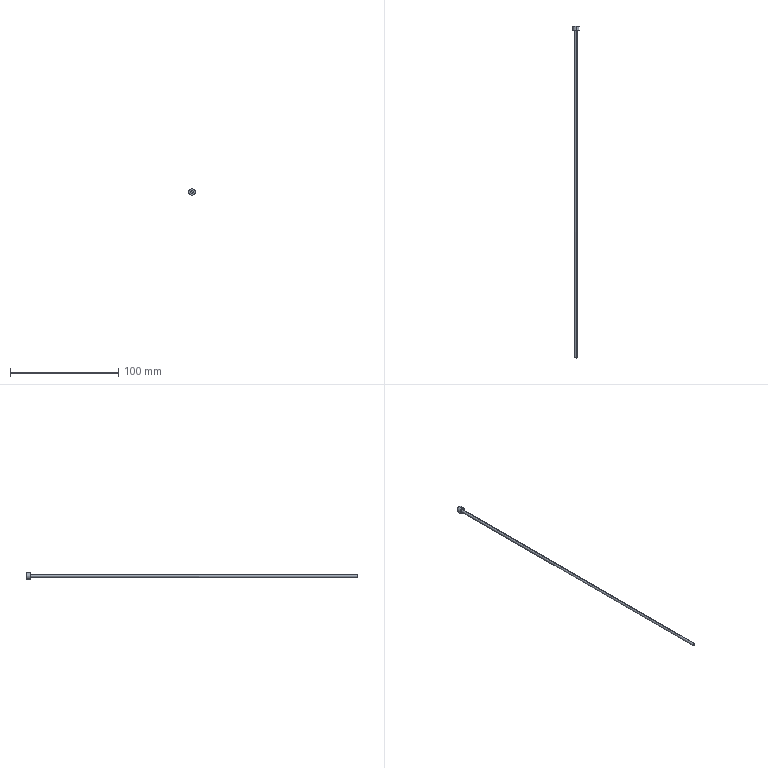Part | STEP file | 1 solid | 7 faces | box 6 x 306.305 x 6 mm | volume 1597 mm3 | cylinder 4 | plane 3 | commonest cylinder face diameters 2.5 x2 6 x2
STEP:
#1=CARTESIAN_POINT('',(0.,0.,0.));
#2=DIRECTION('',(0.,0.,1.));
#3=DIRECTION('',(1.,0.,0.));
#4=AXIS2_PLACEMENT_3D('',#1,#2,#3);
#5=CARTESIAN_POINT('',(-72.862,345.5,129.66));
#6=VERTEX_POINT('',#5);
#7=CARTESIAN_POINT('',(-72.862,345.5,135.66));
#8=VERTEX_POINT('',#7);
#9=CARTESIAN_POINT('',(-72.862,345.5,132.66));
#10=DIRECTION('',(0.,-1.,0.));
#11=DIRECTION('',(0.,0.,-1.));
#12=AXIS2_PLACEMENT_3D('',#9,#10,#11);
#13=CIRCLE('',#12,3.);
#14=CARTESIAN_POINT('',(-72.862,345.5,132.66));
#15=DIRECTION('',(0.,-1.,0.));
#16=DIRECTION('',(0.,0.,-1.));
#17=AXIS2_PLACEMENT_3D('',#14,#15,#16);
#18=CYLINDRICAL_SURFACE('',#17,3.);
#19=CARTESIAN_POINT('',(0.,0.));
#20=DIRECTION('',(1.,0.));
#21=VECTOR('',#20,1.);
#22=LINE('',#19,#21);
#23=(GEOMETRIC_REPRESENTATION_CONTEXT(2)PARAMETRIC_REPRESENTATION_CONTEXT()REPRESENTATION_CONTEXT('',''));
#24=DEFINITIONAL_REPRESENTATION('',(#22),#23);
#25=PCURVE('',#18,#24);
#26=CARTESIAN_POINT('',(-72.862,345.5,110.196));
#27=DIRECTION('',(0.,-1.,0.));
#28=DIRECTION('',(0.,0.,-1.));
#29=AXIS2_PLACEMENT_3D('',#26,#27,#28);
#30=PLANE('',#29);
#31=CARTESIAN_POINT('',(-22.464,-0.000000011));
#32=DIRECTION('',(1.,0.));
#33=AXIS2_PLACEMENT_2D('',#31,#32);
#34=CIRCLE('',#33,3.);
#35=(GEOMETRIC_REPRESENTATION_CONTEXT(2)PARAMETRIC_REPRESENTATION_CONTEXT()REPRESENTATION_CONTEXT('',''));
#36=DEFINITIONAL_REPRESENTATION('',(#34),#35);
#37=PCURVE('',#30,#36);
#38=SURFACE_CURVE('',#13,(#25,#37),.PCURVE_S1.);
#39=EDGE_CURVE('',#6,#8,#38,.T.);
#40=ORIENTED_EDGE('',*,*,#39,.T.);
#41=CARTESIAN_POINT('',(-72.862,341.5,135.66));
#42=VERTEX_POINT('',#41);
#43=CARTESIAN_POINT('',(-72.862,345.5,135.66));
#44=DIRECTION('',(0.,-1.,0.));
#45=VECTOR('',#44,1.);
#46=LINE('',#43,#45);
#47=CARTESIAN_POINT('',(3.142,0.));
#48=DIRECTION('',(0.,1.));
#49=VECTOR('',#48,1.);
#50=LINE('',#47,#49);
#51=(GEOMETRIC_REPRESENTATION_CONTEXT(2)PARAMETRIC_REPRESENTATION_CONTEXT()REPRESENTATION_CONTEXT('',''));
#52=DEFINITIONAL_REPRESENTATION('',(#50),#51);
#53=PCURVE('',#18,#52);
#54=CARTESIAN_POINT('',(-72.862,345.5,132.66));
#55=DIRECTION('',(0.,-1.,0.));
#56=DIRECTION('',(0.,0.,-1.));
#57=AXIS2_PLACEMENT_3D('',#54,#55,#56);
#58=CYLINDRICAL_SURFACE('',#57,3.);
#59=CARTESIAN_POINT('',(3.142,0.));
#60=DIRECTION('',(0.,1.));
#61=VECTOR('',#60,1.);
#62=LINE('',#59,#61);
#63=(GEOMETRIC_REPRESENTATION_CONTEXT(2)PARAMETRIC_REPRESENTATION_CONTEXT()REPRESENTATION_CONTEXT('',''));
#64=DEFINITIONAL_REPRESENTATION('',(#62),#63);
#65=PCURVE('',#58,#64);
#66=SURFACE_CURVE('',#46,(#53,#65),.PCURVE_S1.);
#67=EDGE_CURVE('',#8,#42,#66,.T.);
#68=ORIENTED_EDGE('',*,*,#67,.T.);
#69=CARTESIAN_POINT('',(-72.862,341.5,129.66));
#70=VERTEX_POINT('',#69);
#71=CARTESIAN_POINT('',(-72.862,341.5,132.66));
#72=DIRECTION('',(0.,1.,0.));
#73=DIRECTION('',(0.,0.,1.));
#74=AXIS2_PLACEMENT_3D('',#71,#72,#73);
#75=CIRCLE('',#74,3.);
#76=CARTESIAN_POINT('',(3.142,4.));
#77=DIRECTION('',(-1.,0.));
#78=VECTOR('',#77,1.);
#79=LINE('',#76,#78);
#80=(GEOMETRIC_REPRESENTATION_CONTEXT(2)PARAMETRIC_REPRESENTATION_CONTEXT()REPRESENTATION_CONTEXT('',''));
#81=DEFINITIONAL_REPRESENTATION('',(#79),#80);
#82=PCURVE('',#18,#81);
#83=CARTESIAN_POINT('',(-72.862,341.5,132.66));
#84=DIRECTION('',(0.,-1.,0.));
#85=DIRECTION('',(0.,0.,-1.));
#86=AXIS2_PLACEMENT_3D('',#83,#84,#85);
#87=PLANE('',#86);
#88=CARTESIAN_POINT('',(-3.,0.));
#89=CARTESIAN_POINT('',(-3.,5.196));
#90=CARTESIAN_POINT('',(1.5,2.598));
#91=CARTESIAN_POINT('',(6.,0.));
#92=CARTESIAN_POINT('',(1.5,-2.598));
#93=CARTESIAN_POINT('',(-3.,-5.196));
#94=CARTESIAN_POINT('',(-3.,0.));
#95=(BOUNDED_CURVE()B_SPLINE_CURVE(2,(#88,#89,#90,#91,#92,#93,#94),.UNSPECIFIED.,.T.,.F.)B_SPLINE_CURVE_WITH_KNOTS((1,2,2,2,2,1),(-2.094,0.,2.094,4.189,6.283,8.378),.UNSPECIFIED.)CURVE()GEOMETRIC_REPRESENTATION_ITEM()RATIONAL_B_SPLINE_CURVE((1.,0.5,1.,0.5,1.,0.5,1.))REPRESENTATION_ITEM(''));
#96=(GEOMETRIC_REPRESENTATION_CONTEXT(2)PARAMETRIC_REPRESENTATION_CONTEXT()REPRESENTATION_CONTEXT('',''));
#97=DEFINITIONAL_REPRESENTATION('',(#95),#96);
#98=PCURVE('',#87,#97);
#99=SURFACE_CURVE('',#75,(#82,#98),.PCURVE_S1.);
#100=EDGE_CURVE('',#42,#70,#99,.T.);
#101=ORIENTED_EDGE('',*,*,#100,.T.);
#102=CARTESIAN_POINT('',(-72.862,345.5,129.66));
#103=DIRECTION('',(0.,-1.,0.));
#104=VECTOR('',#103,1.);
#105=LINE('',#102,#104);
#106=CARTESIAN_POINT('',(0.,0.));
#107=DIRECTION('',(0.,1.));
#108=VECTOR('',#107,1.);
#109=LINE('',#106,#108);
#110=(GEOMETRIC_REPRESENTATION_CONTEXT(2)PARAMETRIC_REPRESENTATION_CONTEXT()REPRESENTATION_CONTEXT('',''));
#111=DEFINITIONAL_REPRESENTATION('',(#109),#110);
#112=PCURVE('',#18,#111);
#113=CARTESIAN_POINT('',(6.283,0.));
#114=DIRECTION('',(0.,1.));
#115=VECTOR('',#114,1.);
#116=LINE('',#113,#115);
#117=(GEOMETRIC_REPRESENTATION_CONTEXT(2)PARAMETRIC_REPRESENTATION_CONTEXT()REPRESENTATION_CONTEXT('',''));
#118=DEFINITIONAL_REPRESENTATION('',(#116),#117);
#119=PCURVE('',#58,#118);
#120=SURFACE_CURVE('',#105,(#112,#119),.PCURVE_S1.);
#121=EDGE_CURVE('',#6,#70,#120,.T.);
#122=ORIENTED_EDGE('',*,*,#121,.F.);
#123=EDGE_LOOP('',(#40,#68,#101,#122));
#124=FACE_BOUND('',#123,.T.);
#125=ADVANCED_FACE('',(#124),#18,.T.);
#126=CARTESIAN_POINT('',(-72.862,39.195,133.91));
#127=VERTEX_POINT('',#126);
#128=CARTESIAN_POINT('',(-72.862,39.195,131.41));
#129=VERTEX_POINT('',#128);
#130=CARTESIAN_POINT('',(-72.862,39.195,133.91));
#131=CARTESIAN_POINT('',(-72.699,39.195,133.91));
#132=CARTESIAN_POINT('',(-72.535,39.195,133.877));
#133=CARTESIAN_POINT('',(-72.233,39.195,133.752));
#134=CARTESIAN_POINT('',(-72.094,39.195,133.66));
#135=CARTESIAN_POINT('',(-71.863,39.195,133.428));
#136=CARTESIAN_POINT('',(-71.77,39.195,133.29));
#137=CARTESIAN_POINT('',(-71.645,39.195,132.987));
#138=CARTESIAN_POINT('',(-71.612,39.195,132.824));
#139=CARTESIAN_POINT('',(-71.612,39.195,132.496));
#140=CARTESIAN_POINT('',(-71.645,39.195,132.333));
#141=CARTESIAN_POINT('',(-71.77,39.195,132.03));
#142=CARTESIAN_POINT('',(-71.863,39.195,131.892));
#143=CARTESIAN_POINT('',(-72.094,39.195,131.66));
#144=CARTESIAN_POINT('',(-72.233,39.195,131.568));
#145=CARTESIAN_POINT('',(-72.535,39.195,131.443));
#146=CARTESIAN_POINT('',(-72.699,39.195,131.41));
#147=CARTESIAN_POINT('',(-72.862,39.195,131.41));
#148=B_SPLINE_CURVE_WITH_KNOTS('',3,(#130,#131,#132,#133,#134,#135,#136,#137,#138,#139,#140,#141,#142,#143,#144,#145,#146,#147),.UNSPECIFIED.,.F.,.F.,(4,2,2,2,2,2,2,2,4),(0.,0.0625,0.125,0.1875,0.25,0.3125,0.375,0.4375,0.5),.UNSPECIFIED.);
#149=CARTESIAN_POINT('',(-72.862,39.195,132.66));
#150=DIRECTION('',(0.,1.,0.));
#151=DIRECTION('',(0.,0.,1.));
#152=AXIS2_PLACEMENT_3D('',#149,#150,#151);
#153=CYLINDRICAL_SURFACE('',#152,1.25);
#154=CARTESIAN_POINT('',(0.,0.));
#155=CARTESIAN_POINT('',(3.142,0.));
#156=B_SPLINE_CURVE_WITH_KNOTS('',1,(#154,#155),.UNSPECIFIED.,.F.,.F.,(2,2),(0.,0.5),.PIECEWISE_BEZIER_KNOTS.);
#157=(GEOMETRIC_REPRESENTATION_CONTEXT(2)PARAMETRIC_REPRESENTATION_CONTEXT()REPRESENTATION_CONTEXT('',''));
#158=DEFINITIONAL_REPRESENTATION('',(#156),#157);
#159=PCURVE('',#153,#158);
#160=CARTESIAN_POINT('',(-72.862,39.195,132.66));
#161=DIRECTION('',(0.,-1.,0.));
#162=DIRECTION('',(0.,0.,-1.));
#163=AXIS2_PLACEMENT_3D('',#160,#161,#162);
#164=PLANE('',#163);
#165=CARTESIAN_POINT('',(-1.25,0.));
#166=CARTESIAN_POINT('',(-1.25,0.1636));
#167=CARTESIAN_POINT('',(-1.217,0.3272));
#168=CARTESIAN_POINT('',(-1.092,0.6295));
#169=CARTESIAN_POINT('',(-0.9996,0.7682));
#170=CARTESIAN_POINT('',(-0.7682,0.9996));
#171=CARTESIAN_POINT('',(-0.6295,1.092));
#172=CARTESIAN_POINT('',(-0.3272,1.217));
#173=CARTESIAN_POINT('',(-0.1636,1.25));
#174=CARTESIAN_POINT('',(0.1636,1.25));
#175=CARTESIAN_POINT('',(0.3272,1.217));
#176=CARTESIAN_POINT('',(0.6295,1.092));
#177=CARTESIAN_POINT('',(0.7682,0.9996));
#178=CARTESIAN_POINT('',(0.9996,0.7682));
#179=CARTESIAN_POINT('',(1.092,0.6295));
#180=CARTESIAN_POINT('',(1.217,0.3272));
#181=CARTESIAN_POINT('',(1.25,0.1636));
#182=CARTESIAN_POINT('',(1.25,0.));
#183=B_SPLINE_CURVE_WITH_KNOTS('',3,(#165,#166,#167,#168,#169,#170,#171,#172,#173,#174,#175,#176,#177,#178,#179,#180,#181,#182),.UNSPECIFIED.,.F.,.F.,(4,2,2,2,2,2,2,2,4),(0.,0.0625,0.125,0.1875,0.25,0.3125,0.375,0.4375,0.5),.UNSPECIFIED.);
#184=(GEOMETRIC_REPRESENTATION_CONTEXT(2)PARAMETRIC_REPRESENTATION_CONTEXT()REPRESENTATION_CONTEXT('',''));
#185=DEFINITIONAL_REPRESENTATION('',(#183),#184);
#186=PCURVE('',#164,#185);
#187=SURFACE_CURVE('',#148,(#159,#186),.PCURVE_S1.);
#188=EDGE_CURVE('',#127,#129,#187,.T.);
#189=ORIENTED_EDGE('',*,*,#188,.T.);
#190=CARTESIAN_POINT('',(-72.862,341.5,131.41));
#191=VERTEX_POINT('',#190);
#192=CARTESIAN_POINT('',(-72.862,39.195,131.41));
#193=DIRECTION('',(0.,1.,0.));
#194=VECTOR('',#193,1.);
#195=LINE('',#192,#194);
#196=CARTESIAN_POINT('',(3.142,0.));
#197=DIRECTION('',(0.,1.));
#198=VECTOR('',#197,1.);
#199=LINE('',#196,#198);
#200=(GEOMETRIC_REPRESENTATION_CONTEXT(2)PARAMETRIC_REPRESENTATION_CONTEXT()REPRESENTATION_CONTEXT('',''));
#201=DEFINITIONAL_REPRESENTATION('',(#199),#200);
#202=PCURVE('',#153,#201);
#203=CARTESIAN_POINT('',(-72.862,39.195,132.66));
#204=DIRECTION('',(0.,1.,0.));
#205=DIRECTION('',(0.,0.,1.));
#206=AXIS2_PLACEMENT_3D('',#203,#204,#205);
#207=CYLINDRICAL_SURFACE('',#206,1.25);
#208=CARTESIAN_POINT('',(3.142,0.));
#209=DIRECTION('',(0.,1.));
#210=VECTOR('',#209,1.);
#211=LINE('',#208,#210);
#212=(GEOMETRIC_REPRESENTATION_CONTEXT(2)PARAMETRIC_REPRESENTATION_CONTEXT()REPRESENTATION_CONTEXT('',''));
#213=DEFINITIONAL_REPRESENTATION('',(#211),#212);
#214=PCURVE('',#207,#213);
#215=SURFACE_CURVE('',#195,(#202,#214),.PCURVE_S1.);
#216=EDGE_CURVE('',#129,#191,#215,.T.);
#217=ORIENTED_EDGE('',*,*,#216,.T.);
#218=CARTESIAN_POINT('',(-72.862,341.5,133.91));
#219=VERTEX_POINT('',#218);
#220=CARTESIAN_POINT('',(-72.862,341.5,132.66));
#221=DIRECTION('',(0.,1.,0.));
#222=DIRECTION('',(0.,0.,-1.));
#223=AXIS2_PLACEMENT_3D('',#220,#221,#222);
#224=CIRCLE('',#223,1.25);
#225=CARTESIAN_POINT('',(-3.142,302.305));
#226=DIRECTION('',(1.,0.));
#227=VECTOR('',#226,1.);
#228=LINE('',#225,#227);
#229=(GEOMETRIC_REPRESENTATION_CONTEXT(2)PARAMETRIC_REPRESENTATION_CONTEXT()REPRESENTATION_CONTEXT('',''));
#230=DEFINITIONAL_REPRESENTATION('',(#228),#229);
#231=PCURVE('',#153,#230);
#232=CARTESIAN_POINT('',(1.25,0.));
#233=CARTESIAN_POINT('',(1.25,-2.165));
#234=CARTESIAN_POINT('',(-0.625,-1.083));
#235=CARTESIAN_POINT('',(-2.5,0.));
#236=CARTESIAN_POINT('',(-0.625,1.083));
#237=CARTESIAN_POINT('',(1.25,2.165));
#238=CARTESIAN_POINT('',(1.25,0.));
#239=(BOUNDED_CURVE()B_SPLINE_CURVE(2,(#232,#233,#234,#235,#236,#237,#238),.UNSPECIFIED.,.T.,.F.)B_SPLINE_CURVE_WITH_KNOTS((1,2,2,2,2,1),(-2.094,0.,2.094,4.189,6.283,8.378),.UNSPECIFIED.)CURVE()GEOMETRIC_REPRESENTATION_ITEM()RATIONAL_B_SPLINE_CURVE((1.,0.5,1.,0.5,1.,0.5,1.))REPRESENTATION_ITEM(''));
#240=(GEOMETRIC_REPRESENTATION_CONTEXT(2)PARAMETRIC_REPRESENTATION_CONTEXT()REPRESENTATION_CONTEXT('',''));
#241=DEFINITIONAL_REPRESENTATION('',(#239),#240);
#242=PCURVE('',#87,#241);
#243=SURFACE_CURVE('',#224,(#231,#242),.PCURVE_S1.);
#244=EDGE_CURVE('',#219,#191,#243,.T.);
#245=ORIENTED_EDGE('',*,*,#244,.F.);
#246=CARTESIAN_POINT('',(-72.862,39.195,133.91));
#247=DIRECTION('',(0.,1.,0.));
#248=VECTOR('',#247,1.);
#249=LINE('',#246,#248);
#250=CARTESIAN_POINT('',(0.,0.));
#251=DIRECTION('',(0.,1.));
#252=VECTOR('',#251,1.);
#253=LINE('',#250,#252);
#254=(GEOMETRIC_REPRESENTATION_CONTEXT(2)PARAMETRIC_REPRESENTATION_CONTEXT()REPRESENTATION_CONTEXT('',''));
#255=DEFINITIONAL_REPRESENTATION('',(#253),#254);
#256=PCURVE('',#153,#255);
#257=CARTESIAN_POINT('',(6.283,0.));
#258=DIRECTION('',(0.,1.));
#259=VECTOR('',#258,1.);
#260=LINE('',#257,#259);
#261=(GEOMETRIC_REPRESENTATION_CONTEXT(2)PARAMETRIC_REPRESENTATION_CONTEXT()REPRESENTATION_CONTEXT('',''));
#262=DEFINITIONAL_REPRESENTATION('',(#260),#261);
#263=PCURVE('',#207,#262);
#264=SURFACE_CURVE('',#249,(#256,#263),.PCURVE_S1.);
#265=EDGE_CURVE('',#127,#219,#264,.T.);
#266=ORIENTED_EDGE('',*,*,#265,.F.);
#267=EDGE_LOOP('',(#189,#217,#245,#266));
#268=FACE_BOUND('',#267,.T.);
#269=ADVANCED_FACE('',(#268),#153,.T.);
#270=ORIENTED_EDGE('',*,*,#216,.F.);
#271=CARTESIAN_POINT('',(-72.862,39.195,131.41));
#272=CARTESIAN_POINT('',(-73.026,39.195,131.41));
#273=CARTESIAN_POINT('',(-73.19,39.195,131.443));
#274=CARTESIAN_POINT('',(-73.492,39.195,131.568));
#275=CARTESIAN_POINT('',(-73.631,39.195,131.66));
#276=CARTESIAN_POINT('',(-73.862,39.195,131.892));
#277=CARTESIAN_POINT('',(-73.955,39.195,132.03));
#278=CARTESIAN_POINT('',(-74.08,39.195,132.333));
#279=CARTESIAN_POINT('',(-74.112,39.195,132.496));
#280=CARTESIAN_POINT('',(-74.112,39.195,132.824));
#281=CARTESIAN_POINT('',(-74.08,39.195,132.987));
#282=CARTESIAN_POINT('',(-73.955,39.195,133.29));
#283=CARTESIAN_POINT('',(-73.862,39.195,133.428));
#284=CARTESIAN_POINT('',(-73.631,39.195,133.66));
#285=CARTESIAN_POINT('',(-73.492,39.195,133.752));
#286=CARTESIAN_POINT('',(-73.19,39.195,133.877));
#287=CARTESIAN_POINT('',(-73.026,39.195,133.91));
#288=CARTESIAN_POINT('',(-72.862,39.195,133.91));
#289=B_SPLINE_CURVE_WITH_KNOTS('',3,(#271,#272,#273,#274,#275,#276,#277,#278,#279,#280,#281,#282,#283,#284,#285,#286,#287,#288),.UNSPECIFIED.,.F.,.F.,(4,2,2,2,2,2,2,2,4),(0.5,0.5625,0.625,0.6875,0.75,0.8125,0.875,0.9375,1.),.UNSPECIFIED.);
#290=CARTESIAN_POINT('',(3.142,0.));
#291=CARTESIAN_POINT('',(6.283,0.));
#292=B_SPLINE_CURVE_WITH_KNOTS('',1,(#290,#291),.UNSPECIFIED.,.F.,.F.,(2,2),(0.5,1.),.PIECEWISE_BEZIER_KNOTS.);
#293=(GEOMETRIC_REPRESENTATION_CONTEXT(2)PARAMETRIC_REPRESENTATION_CONTEXT()REPRESENTATION_CONTEXT('',''));
#294=DEFINITIONAL_REPRESENTATION('',(#292),#293);
#295=PCURVE('',#207,#294);
#296=CARTESIAN_POINT('',(1.25,0.));
#297=CARTESIAN_POINT('',(1.25,-0.1636));
#298=CARTESIAN_POINT('',(1.217,-0.3272));
#299=CARTESIAN_POINT('',(1.092,-0.6295));
#300=CARTESIAN_POINT('',(0.9996,-0.7682));
#301=CARTESIAN_POINT('',(0.7682,-0.9996));
#302=CARTESIAN_POINT('',(0.6295,-1.092));
#303=CARTESIAN_POINT('',(0.3272,-1.217));
#304=CARTESIAN_POINT('',(0.1636,-1.25));
#305=CARTESIAN_POINT('',(-0.1636,-1.25));
#306=CARTESIAN_POINT('',(-0.3272,-1.217));
#307=CARTESIAN_POINT('',(-0.6295,-1.092));
#308=CARTESIAN_POINT('',(-0.7682,-0.9996));
#309=CARTESIAN_POINT('',(-0.9996,-0.7682));
#310=CARTESIAN_POINT('',(-1.092,-0.6295));
#311=CARTESIAN_POINT('',(-1.217,-0.3272));
#312=CARTESIAN_POINT('',(-1.25,-0.1636));
#313=CARTESIAN_POINT('',(-1.25,0.));
#314=B_SPLINE_CURVE_WITH_KNOTS('',3,(#296,#297,#298,#299,#300,#301,#302,#303,#304,#305,#306,#307,#308,#309,#310,#311,#312,#313),.UNSPECIFIED.,.F.,.F.,(4,2,2,2,2,2,2,2,4),(0.5,0.5625,0.625,0.6875,0.75,0.8125,0.875,0.9375,1.),.UNSPECIFIED.);
#315=(GEOMETRIC_REPRESENTATION_CONTEXT(2)PARAMETRIC_REPRESENTATION_CONTEXT()REPRESENTATION_CONTEXT('',''));
#316=DEFINITIONAL_REPRESENTATION('',(#314),#315);
#317=PCURVE('',#164,#316);
#318=SURFACE_CURVE('',#289,(#295,#317),.PCURVE_S1.);
#319=EDGE_CURVE('',#129,#127,#318,.T.);
#320=ORIENTED_EDGE('',*,*,#319,.T.);
#321=ORIENTED_EDGE('',*,*,#265,.T.);
#322=CARTESIAN_POINT('',(-72.862,341.5,132.66));
#323=DIRECTION('',(0.,1.,0.));
#324=DIRECTION('',(0.,0.,-1.));
#325=AXIS2_PLACEMENT_3D('',#322,#323,#324);
#326=CIRCLE('',#325,1.25);
#327=CARTESIAN_POINT('',(3.142,302.305));
#328=DIRECTION('',(1.,0.));
#329=VECTOR('',#328,1.);
#330=LINE('',#327,#329);
#331=(GEOMETRIC_REPRESENTATION_CONTEXT(2)PARAMETRIC_REPRESENTATION_CONTEXT()REPRESENTATION_CONTEXT('',''));
#332=DEFINITIONAL_REPRESENTATION('',(#330),#331);
#333=PCURVE('',#207,#332);
#334=CARTESIAN_POINT('',(1.25,0.));
#335=CARTESIAN_POINT('',(1.25,-2.165));
#336=CARTESIAN_POINT('',(-0.625,-1.083));
#337=CARTESIAN_POINT('',(-2.5,0.));
#338=CARTESIAN_POINT('',(-0.625,1.083));
#339=CARTESIAN_POINT('',(1.25,2.165));
#340=CARTESIAN_POINT('',(1.25,0.));
#341=(BOUNDED_CURVE()B_SPLINE_CURVE(2,(#334,#335,#336,#337,#338,#339,#340),.UNSPECIFIED.,.T.,.F.)B_SPLINE_CURVE_WITH_KNOTS((1,2,2,2,2,1),(-2.094,0.,2.094,4.189,6.283,8.378),.UNSPECIFIED.)CURVE()GEOMETRIC_REPRESENTATION_ITEM()RATIONAL_B_SPLINE_CURVE((1.,0.5,1.,0.5,1.,0.5,1.))REPRESENTATION_ITEM(''));
#342=(GEOMETRIC_REPRESENTATION_CONTEXT(2)PARAMETRIC_REPRESENTATION_CONTEXT()REPRESENTATION_CONTEXT('',''));
#343=DEFINITIONAL_REPRESENTATION('',(#341),#342);
#344=PCURVE('',#87,#343);
#345=SURFACE_CURVE('',#326,(#333,#344),.PCURVE_S1.);
#346=EDGE_CURVE('',#191,#219,#345,.T.);
#347=ORIENTED_EDGE('',*,*,#346,.F.);
#348=EDGE_LOOP('',(#270,#320,#321,#347));
#349=FACE_BOUND('',#348,.T.);
#350=ADVANCED_FACE('',(#349),#207,.T.);
#351=ORIENTED_EDGE('',*,*,#188,.F.);
#352=ORIENTED_EDGE('',*,*,#319,.F.);
#353=EDGE_LOOP('',(#351,#352));
#354=FACE_BOUND('',#353,.T.);
#355=ADVANCED_FACE('',(#354),#164,.T.);
#356=ORIENTED_EDGE('',*,*,#244,.T.);
#357=ORIENTED_EDGE('',*,*,#346,.T.);
#358=EDGE_LOOP('',(#356,#357));
#359=FACE_BOUND('',#358,.T.);
#360=CARTESIAN_POINT('',(-72.862,341.5,132.66));
#361=DIRECTION('',(0.,1.,0.));
#362=DIRECTION('',(0.,0.,1.));
#363=AXIS2_PLACEMENT_3D('',#360,#361,#362);
#364=CIRCLE('',#363,3.);
#365=CARTESIAN_POINT('',(-3.,0.));
#366=CARTESIAN_POINT('',(-3.,5.196));
#367=CARTESIAN_POINT('',(1.5,2.598));
#368=CARTESIAN_POINT('',(6.,0.));
#369=CARTESIAN_POINT('',(1.5,-2.598));
#370=CARTESIAN_POINT('',(-3.,-5.196));
#371=CARTESIAN_POINT('',(-3.,0.));
#372=(BOUNDED_CURVE()B_SPLINE_CURVE(2,(#365,#366,#367,#368,#369,#370,#371),.UNSPECIFIED.,.T.,.F.)B_SPLINE_CURVE_WITH_KNOTS((1,2,2,2,2,1),(-2.094,0.,2.094,4.189,6.283,8.378),.UNSPECIFIED.)CURVE()GEOMETRIC_REPRESENTATION_ITEM()RATIONAL_B_SPLINE_CURVE((1.,0.5,1.,0.5,1.,0.5,1.))REPRESENTATION_ITEM(''));
#373=(GEOMETRIC_REPRESENTATION_CONTEXT(2)PARAMETRIC_REPRESENTATION_CONTEXT()REPRESENTATION_CONTEXT('',''));
#374=DEFINITIONAL_REPRESENTATION('',(#372),#373);
#375=PCURVE('',#87,#374);
#376=CARTESIAN_POINT('',(9.425,4.));
#377=DIRECTION('',(-1.,0.));
#378=VECTOR('',#377,1.);
#379=LINE('',#376,#378);
#380=(GEOMETRIC_REPRESENTATION_CONTEXT(2)PARAMETRIC_REPRESENTATION_CONTEXT()REPRESENTATION_CONTEXT('',''));
#381=DEFINITIONAL_REPRESENTATION('',(#379),#380);
#382=PCURVE('',#58,#381);
#383=SURFACE_CURVE('',#364,(#375,#382),.PCURVE_S1.);
#384=EDGE_CURVE('',#70,#42,#383,.T.);
#385=ORIENTED_EDGE('',*,*,#384,.F.);
#386=ORIENTED_EDGE('',*,*,#100,.F.);
#387=EDGE_LOOP('',(#385,#386));
#388=FACE_BOUND('',#387,.T.);
#389=ADVANCED_FACE('',(#359,#388),#87,.T.);
#390=ORIENTED_EDGE('',*,*,#67,.F.);
#391=CARTESIAN_POINT('',(-72.862,345.5,132.66));
#392=DIRECTION('',(0.,-1.,0.));
#393=DIRECTION('',(0.,0.,-1.));
#394=AXIS2_PLACEMENT_3D('',#391,#392,#393);
#395=CIRCLE('',#394,3.);
#396=CARTESIAN_POINT('',(0.,0.));
#397=DIRECTION('',(1.,0.));
#398=VECTOR('',#397,1.);
#399=LINE('',#396,#398);
#400=(GEOMETRIC_REPRESENTATION_CONTEXT(2)PARAMETRIC_REPRESENTATION_CONTEXT()REPRESENTATION_CONTEXT('',''));
#401=DEFINITIONAL_REPRESENTATION('',(#399),#400);
#402=PCURVE('',#58,#401);
#403=CARTESIAN_POINT('',(-22.464,-0.000000011));
#404=DIRECTION('',(1.,0.));
#405=AXIS2_PLACEMENT_2D('',#403,#404);
#406=CIRCLE('',#405,3.);
#407=(GEOMETRIC_REPRESENTATION_CONTEXT(2)PARAMETRIC_REPRESENTATION_CONTEXT()REPRESENTATION_CONTEXT('',''));
#408=DEFINITIONAL_REPRESENTATION('',(#406),#407);
#409=PCURVE('',#30,#408);
#410=SURFACE_CURVE('',#395,(#402,#409),.PCURVE_S1.);
#411=EDGE_CURVE('',#8,#6,#410,.T.);
#412=ORIENTED_EDGE('',*,*,#411,.T.);
#413=ORIENTED_EDGE('',*,*,#121,.T.);
#414=ORIENTED_EDGE('',*,*,#384,.T.);
#415=EDGE_LOOP('',(#390,#412,#413,#414));
#416=FACE_BOUND('',#415,.T.);
#417=ADVANCED_FACE('',(#416),#58,.T.);
#418=ORIENTED_EDGE('',*,*,#39,.F.);
#419=ORIENTED_EDGE('',*,*,#411,.F.);
#420=EDGE_LOOP('',(#418,#419));
#421=FACE_BOUND('',#420,.T.);
#422=ADVANCED_FACE('',(#421),#30,.F.);
#423=CLOSED_SHELL('',(#125,#269,#350,#355,#389,#417,#422));
#424=MANIFOLD_SOLID_BREP('',#423);
#425=(LENGTH_UNIT()NAMED_UNIT(*)SI_UNIT(.MILLI.,.METRE.));
#426=UNCERTAINTY_MEASURE_WITH_UNIT(LENGTH_MEASURE(0.00002),#425,'','');
#427=(NAMED_UNIT(*)PLANE_ANGLE_UNIT()SI_UNIT($,.RADIAN.));
#428=(NAMED_UNIT(*)SI_UNIT($,.STERADIAN.)SOLID_ANGLE_UNIT());
#429=(GEOMETRIC_REPRESENTATION_CONTEXT(3)GLOBAL_UNCERTAINTY_ASSIGNED_CONTEXT((#426))GLOBAL_UNIT_ASSIGNED_CONTEXT((#425,#427,#428))REPRESENTATION_CONTEXT('',''));
#430=ADVANCED_BREP_SHAPE_REPRESENTATION('',(#4,#424),#429);